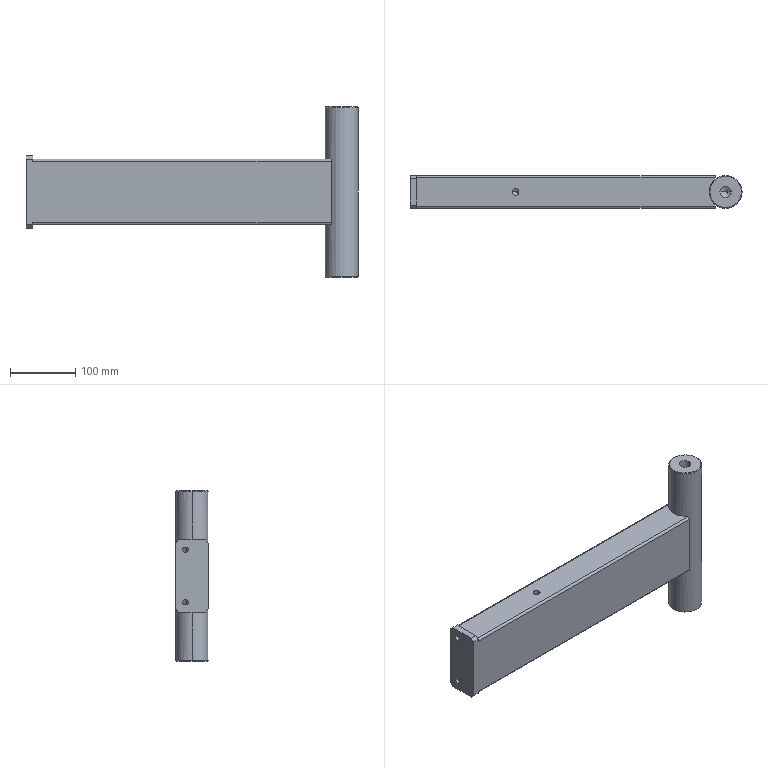Part | SolidWorks | features HoleWzd 6, ICE 3, Chamfer 2, Revolution 2, Extrusion 1, Fillet 1 | 1 solid | 54 faces | box 507 x 50 x 260 mm | volume 953629 mm3 | plane 22 | cylinder 20 | cone 12 | commonest cylinder face diameters 6 x4 8.5 x4 10.2 x4 17.5 x4 20 x2 50 x2